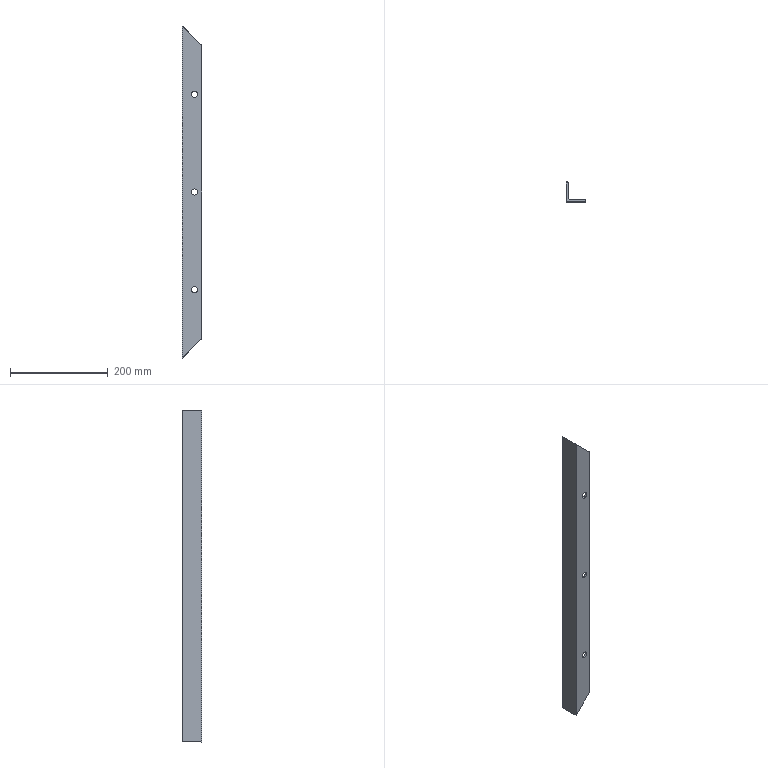Part | SolidWorks | features ICE 2, Extrusion 1 | 1 solid | 17 faces | box 40 x 40 x 680 mm | volume 199359 mm3 | cylinder 9 | plane 8 | commonest cylinder face diameters 13 x6 4 x2 8 x1
STEP:
#1=CARTESIAN_POINT('',(31.5,0.,540.));
#2=VERTEX_POINT('',#1);
#3=CARTESIAN_POINT('',(18.5,0.,540.));
#4=VERTEX_POINT('',#3);
#5=CARTESIAN_POINT('',(25.,0.,540.));
#6=DIRECTION('',(0.,1.,0.));
#7=DIRECTION('',(0.,0.,1.));
#8=AXIS2_PLACEMENT_3D('',#5,#6,#7);
#9=CIRCLE('',#8,6.5);
#10=EDGE_CURVE('',#2,#4,#9,.T.);
#11=ORIENTED_EDGE('',*,*,#10,.F.);
#12=CARTESIAN_POINT('',(31.5,4.,540.));
#13=VERTEX_POINT('',#12);
#14=CARTESIAN_POINT('',(31.5,-6.,540.));
#15=DIRECTION('',(0.,1.,0.));
#16=VECTOR('',#15,1000.);
#17=LINE('',#14,#16);
#18=EDGE_CURVE('',#2,#13,#17,.T.);
#19=ORIENTED_EDGE('',*,*,#18,.T.);
#20=CARTESIAN_POINT('',(18.5,4.,540.));
#21=VERTEX_POINT('',#20);
#22=CARTESIAN_POINT('',(25.,4.,540.));
#23=DIRECTION('',(0.,1.,0.));
#24=DIRECTION('',(-1.,0.,0.));
#25=AXIS2_PLACEMENT_3D('',#22,#23,#24);
#26=CIRCLE('',#25,6.5);
#27=EDGE_CURVE('',#13,#21,#26,.T.);
#28=ORIENTED_EDGE('',*,*,#27,.T.);
#29=CARTESIAN_POINT('',(18.5,-6.,540.));
#30=DIRECTION('',(0.,1.,0.));
#31=VECTOR('',#30,1000.);
#32=LINE('',#29,#31);
#33=EDGE_CURVE('',#4,#21,#32,.T.);
#34=ORIENTED_EDGE('',*,*,#33,.F.);
#35=EDGE_LOOP('',(#11,#19,#28,#34));
#36=FACE_OUTER_BOUND('',#35,.T.);
#37=CARTESIAN_POINT('',(25.,-6.,540.));
#38=DIRECTION('',(0.,1.,0.));
#39=DIRECTION('',(-1.,0.,0.));
#40=AXIS2_PLACEMENT_3D('',#37,#38,#39);
#41=CYLINDRICAL_SURFACE('',#40,6.5);
#42=ADVANCED_FACE('',(#36),#41,.F.);
#43=CARTESIAN_POINT('',(31.5,0.,340.));
#44=VERTEX_POINT('',#43);
#45=CARTESIAN_POINT('',(18.5,0.,340.));
#46=VERTEX_POINT('',#45);
#47=CARTESIAN_POINT('',(25.,0.,340.));
#48=DIRECTION('',(0.,1.,0.));
#49=DIRECTION('',(0.,0.,1.));
#50=AXIS2_PLACEMENT_3D('',#47,#48,#49);
#51=CIRCLE('',#50,6.5);
#52=EDGE_CURVE('',#44,#46,#51,.T.);
#53=ORIENTED_EDGE('',*,*,#52,.F.);
#54=CARTESIAN_POINT('',(31.5,4.,340.));
#55=VERTEX_POINT('',#54);
#56=CARTESIAN_POINT('',(31.5,-6.,340.));
#57=DIRECTION('',(0.,1.,0.));
#58=VECTOR('',#57,1000.);
#59=LINE('',#56,#58);
#60=EDGE_CURVE('',#44,#55,#59,.T.);
#61=ORIENTED_EDGE('',*,*,#60,.T.);
#62=CARTESIAN_POINT('',(18.5,4.,340.));
#63=VERTEX_POINT('',#62);
#64=CARTESIAN_POINT('',(25.,4.,340.));
#65=DIRECTION('',(0.,1.,0.));
#66=DIRECTION('',(-1.,0.,0.));
#67=AXIS2_PLACEMENT_3D('',#64,#65,#66);
#68=CIRCLE('',#67,6.5);
#69=EDGE_CURVE('',#55,#63,#68,.T.);
#70=ORIENTED_EDGE('',*,*,#69,.T.);
#71=CARTESIAN_POINT('',(18.5,-6.,340.));
#72=DIRECTION('',(0.,1.,0.));
#73=VECTOR('',#72,1000.);
#74=LINE('',#71,#73);
#75=EDGE_CURVE('',#46,#63,#74,.T.);
#76=ORIENTED_EDGE('',*,*,#75,.F.);
#77=EDGE_LOOP('',(#53,#61,#70,#76));
#78=FACE_OUTER_BOUND('',#77,.T.);
#79=CARTESIAN_POINT('',(25.,-6.,340.));
#80=DIRECTION('',(0.,1.,0.));
#81=DIRECTION('',(-1.,0.,0.));
#82=AXIS2_PLACEMENT_3D('',#79,#80,#81);
#83=CYLINDRICAL_SURFACE('',#82,6.5);
#84=ADVANCED_FACE('',(#78),#83,.F.);
#85=CARTESIAN_POINT('',(31.5,0.,140.));
#86=VERTEX_POINT('',#85);
#87=CARTESIAN_POINT('',(18.5,0.,140.));
#88=VERTEX_POINT('',#87);
#89=CARTESIAN_POINT('',(25.,0.,140.));
#90=DIRECTION('',(0.,1.,0.));
#91=DIRECTION('',(0.,0.,1.));
#92=AXIS2_PLACEMENT_3D('',#89,#90,#91);
#93=CIRCLE('',#92,6.5);
#94=EDGE_CURVE('',#86,#88,#93,.T.);
#95=ORIENTED_EDGE('',*,*,#94,.F.);
#96=CARTESIAN_POINT('',(31.5,4.,140.));
#97=VERTEX_POINT('',#96);
#98=CARTESIAN_POINT('',(31.5,-6.,140.));
#99=DIRECTION('',(0.,1.,0.));
#100=VECTOR('',#99,1000.);
#101=LINE('',#98,#100);
#102=EDGE_CURVE('',#86,#97,#101,.T.);
#103=ORIENTED_EDGE('',*,*,#102,.T.);
#104=CARTESIAN_POINT('',(18.5,4.,140.));
#105=VERTEX_POINT('',#104);
#106=CARTESIAN_POINT('',(25.,4.,140.));
#107=DIRECTION('',(0.,1.,0.));
#108=DIRECTION('',(-1.,0.,0.));
#109=AXIS2_PLACEMENT_3D('',#106,#107,#108);
#110=CIRCLE('',#109,6.5);
#111=EDGE_CURVE('',#97,#105,#110,.T.);
#112=ORIENTED_EDGE('',*,*,#111,.T.);
#113=CARTESIAN_POINT('',(18.5,-6.,140.));
#114=DIRECTION('',(0.,1.,0.));
#115=VECTOR('',#114,1000.);
#116=LINE('',#113,#115);
#117=EDGE_CURVE('',#88,#105,#116,.T.);
#118=ORIENTED_EDGE('',*,*,#117,.F.);
#119=EDGE_LOOP('',(#95,#103,#112,#118));
#120=FACE_OUTER_BOUND('',#119,.T.);
#121=CARTESIAN_POINT('',(25.,-6.,140.));
#122=DIRECTION('',(0.,1.,0.));
#123=DIRECTION('',(-1.,0.,0.));
#124=AXIS2_PLACEMENT_3D('',#121,#122,#123);
#125=CYLINDRICAL_SURFACE('',#124,6.5);
#126=ADVANCED_FACE('',(#120),#125,.F.);
#127=CARTESIAN_POINT('',(0.,40.,680.));
#128=VERTEX_POINT('',#127);
#129=CARTESIAN_POINT('',(0.,40.,0.));
#130=VERTEX_POINT('',#129);
#131=CARTESIAN_POINT('',(0.,40.,680.));
#132=DIRECTION('',(0.,0.,-1.));
#133=VECTOR('',#132,1000.);
#134=LINE('',#131,#133);
#135=EDGE_CURVE('',#128,#130,#134,.T.);
#136=ORIENTED_EDGE('',*,*,#135,.F.);
#137=CARTESIAN_POINT('',(2.,40.,678.));
#138=VERTEX_POINT('',#137);
#139=CARTESIAN_POINT('',(40.,40.,640.));
#140=DIRECTION('',(-0.7071,0.,0.7071));
#141=VECTOR('',#140,1000.);
#142=LINE('',#139,#141);
#143=EDGE_CURVE('',#138,#128,#142,.T.);
#144=ORIENTED_EDGE('',*,*,#143,.F.);
#145=CARTESIAN_POINT('',(2.,40.,2.));
#146=VERTEX_POINT('',#145);
#147=CARTESIAN_POINT('',(2.,40.,680.));
#148=DIRECTION('',(0.,0.,-1.));
#149=VECTOR('',#148,1000.);
#150=LINE('',#147,#149);
#151=EDGE_CURVE('',#138,#146,#150,.T.);
#152=ORIENTED_EDGE('',*,*,#151,.T.);
#153=CARTESIAN_POINT('',(0.,40.,0.));
#154=DIRECTION('',(0.7071,0.,0.7071));
#155=VECTOR('',#154,1000.);
#156=LINE('',#153,#155);
#157=EDGE_CURVE('',#130,#146,#156,.T.);
#158=ORIENTED_EDGE('',*,*,#157,.F.);
#159=EDGE_LOOP('',(#136,#144,#152,#158));
#160=FACE_OUTER_BOUND('',#159,.T.);
#161=CARTESIAN_POINT('',(2.,40.,680.));
#162=DIRECTION('',(0.,-1.,0.));
#163=DIRECTION('',(0.,0.,-1.));
#164=AXIS2_PLACEMENT_3D('',#161,#162,#163);
#165=PLANE('',#164);
#166=ADVANCED_FACE('',(#160),#165,.F.);
#167=CARTESIAN_POINT('',(0.,0.,0.));
#168=VERTEX_POINT('',#167);
#169=CARTESIAN_POINT('',(0.,40.,0.));
#170=DIRECTION('',(0.,-1.,0.));
#171=VECTOR('',#170,1000.);
#172=LINE('',#169,#171);
#173=EDGE_CURVE('',#130,#168,#172,.T.);
#174=ORIENTED_EDGE('',*,*,#173,.T.);
#175=CARTESIAN_POINT('',(0.,0.,680.));
#176=VERTEX_POINT('',#175);
#177=CARTESIAN_POINT('',(0.,0.,680.));
#178=DIRECTION('',(0.,0.,-1.));
#179=VECTOR('',#178,1000.);
#180=LINE('',#177,#179);
#181=EDGE_CURVE('',#176,#168,#180,.T.);
#182=ORIENTED_EDGE('',*,*,#181,.F.);
#183=CARTESIAN_POINT('',(0.,40.,680.));
#184=DIRECTION('',(0.,-1.,0.));
#185=VECTOR('',#184,1000.);
#186=LINE('',#183,#185);
#187=EDGE_CURVE('',#128,#176,#186,.T.);
#188=ORIENTED_EDGE('',*,*,#187,.F.);
#189=ORIENTED_EDGE('',*,*,#135,.T.);
#190=EDGE_LOOP('',(#174,#182,#188,#189));
#191=FACE_OUTER_BOUND('',#190,.T.);
#192=CARTESIAN_POINT('',(0.,40.,680.));
#193=DIRECTION('',(1.,0.,0.));
#194=DIRECTION('',(0.,1.,0.));
#195=AXIS2_PLACEMENT_3D('',#192,#193,#194);
#196=PLANE('',#195);
#197=ADVANCED_FACE('',(#191),#196,.F.);
#198=CARTESIAN_POINT('',(25.,0.,540.));
#199=DIRECTION('',(0.,1.,0.));
#200=DIRECTION('',(0.,0.,1.));
#201=AXIS2_PLACEMENT_3D('',#198,#199,#200);
#202=CIRCLE('',#201,6.5);
#203=EDGE_CURVE('',#4,#2,#202,.T.);
#204=ORIENTED_EDGE('',*,*,#203,.T.);
#205=ORIENTED_EDGE('',*,*,#10,.T.);
#206=EDGE_LOOP('',(#204,#205));
#207=FACE_BOUND('',#206,.T.);
#208=CARTESIAN_POINT('',(25.,0.,340.));
#209=DIRECTION('',(0.,1.,0.));
#210=DIRECTION('',(0.,0.,1.));
#211=AXIS2_PLACEMENT_3D('',#208,#209,#210);
#212=CIRCLE('',#211,6.5);
#213=EDGE_CURVE('',#46,#44,#212,.T.);
#214=ORIENTED_EDGE('',*,*,#213,.T.);
#215=ORIENTED_EDGE('',*,*,#52,.T.);
#216=EDGE_LOOP('',(#214,#215));
#217=FACE_BOUND('',#216,.T.);
#218=CARTESIAN_POINT('',(25.,0.,140.));
#219=DIRECTION('',(0.,1.,0.));
#220=DIRECTION('',(0.,0.,1.));
#221=AXIS2_PLACEMENT_3D('',#218,#219,#220);
#222=CIRCLE('',#221,6.5);
#223=EDGE_CURVE('',#88,#86,#222,.T.);
#224=ORIENTED_EDGE('',*,*,#223,.T.);
#225=ORIENTED_EDGE('',*,*,#94,.T.);
#226=EDGE_LOOP('',(#224,#225));
#227=FACE_BOUND('',#226,.T.);
#228=CARTESIAN_POINT('',(40.,0.,640.));
#229=VERTEX_POINT('',#228);
#230=CARTESIAN_POINT('',(40.,0.,40.));
#231=VERTEX_POINT('',#230);
#232=CARTESIAN_POINT('',(40.,0.,680.));
#233=DIRECTION('',(0.,0.,-1.));
#234=VECTOR('',#233,1000.);
#235=LINE('',#232,#234);
#236=EDGE_CURVE('',#229,#231,#235,.T.);
#237=ORIENTED_EDGE('',*,*,#236,.F.);
#238=CARTESIAN_POINT('',(40.,0.,640.));
#239=DIRECTION('',(-0.7071,0.,0.7071));
#240=VECTOR('',#239,1000.);
#241=LINE('',#238,#240);
#242=EDGE_CURVE('',#229,#176,#241,.T.);
#243=ORIENTED_EDGE('',*,*,#242,.T.);
#244=ORIENTED_EDGE('',*,*,#181,.T.);
#245=CARTESIAN_POINT('',(0.,0.,0.));
#246=DIRECTION('',(0.7071,0.,0.7071));
#247=VECTOR('',#246,1000.);
#248=LINE('',#245,#247);
#249=EDGE_CURVE('',#168,#231,#248,.T.);
#250=ORIENTED_EDGE('',*,*,#249,.T.);
#251=EDGE_LOOP('',(#237,#243,#244,#250));
#252=FACE_OUTER_BOUND('',#251,.T.);
#253=CARTESIAN_POINT('',(0.,0.,680.));
#254=DIRECTION('',(0.,1.,0.));
#255=DIRECTION('',(0.,0.,1.));
#256=AXIS2_PLACEMENT_3D('',#253,#254,#255);
#257=PLANE('',#256);
#258=ADVANCED_FACE('',(#207,#217,#227,#252),#257,.F.);
#259=CARTESIAN_POINT('',(40.,2.,640.));
#260=VERTEX_POINT('',#259);
#261=CARTESIAN_POINT('',(40.,2.,40.));
#262=VERTEX_POINT('',#261);
#263=CARTESIAN_POINT('',(40.,2.,680.));
#264=DIRECTION('',(0.,0.,-1.));
#265=VECTOR('',#264,1000.);
#266=LINE('',#263,#265);
#267=EDGE_CURVE('',#260,#262,#266,.T.);
#268=ORIENTED_EDGE('',*,*,#267,.F.);
#269=CARTESIAN_POINT('',(40.,0.,640.));
#270=DIRECTION('',(0.,1.,0.));
#271=VECTOR('',#270,1000.);
#272=LINE('',#269,#271);
#273=EDGE_CURVE('',#229,#260,#272,.T.);
#274=ORIENTED_EDGE('',*,*,#273,.F.);
#275=ORIENTED_EDGE('',*,*,#236,.T.);
#276=CARTESIAN_POINT('',(40.,0.,40.));
#277=DIRECTION('',(0.,1.,0.));
#278=VECTOR('',#277,1000.);
#279=LINE('',#276,#278);
#280=EDGE_CURVE('',#231,#262,#279,.T.);
#281=ORIENTED_EDGE('',*,*,#280,.T.);
#282=EDGE_LOOP('',(#268,#274,#275,#281));
#283=FACE_OUTER_BOUND('',#282,.T.);
#284=CARTESIAN_POINT('',(40.,0.,680.));
#285=DIRECTION('',(-1.,0.,0.));
#286=DIRECTION('',(0.,0.,1.));
#287=AXIS2_PLACEMENT_3D('',#284,#285,#286);
#288=PLANE('',#287);
#289=ADVANCED_FACE('',(#283),#288,.F.);
#290=CARTESIAN_POINT('',(38.,4.,642.));
#291=VERTEX_POINT('',#290);
#292=CARTESIAN_POINT('',(38.,4.,38.));
#293=VERTEX_POINT('',#292);
#294=CARTESIAN_POINT('',(38.,4.,680.));
#295=DIRECTION('',(0.,0.,-1.));
#296=VECTOR('',#295,1000.);
#297=LINE('',#294,#296);
#298=EDGE_CURVE('',#291,#293,#297,.T.);
#299=ORIENTED_EDGE('',*,*,#298,.F.);
#300=CARTESIAN_POINT('',(38.,4.,642.));
#301=CARTESIAN_POINT('',(39.172,4.,640.828));
#302=CARTESIAN_POINT('',(40.,3.172,640.));
#303=CARTESIAN_POINT('',(40.,2.,640.));
#304=(BOUNDED_CURVE()B_SPLINE_CURVE(3,(#300,#301,#302,#303),.UNSPECIFIED.,.F.,.F.)B_SPLINE_CURVE_WITH_KNOTS((4,4),(4.712,6.283),.UNSPECIFIED.)CURVE()GEOMETRIC_REPRESENTATION_ITEM()RATIONAL_B_SPLINE_CURVE((1.,0.8047,0.8047,1.))REPRESENTATION_ITEM(''));
#305=EDGE_CURVE('',#291,#260,#304,.T.);
#306=ORIENTED_EDGE('',*,*,#305,.T.);
#307=ORIENTED_EDGE('',*,*,#267,.T.);
#308=CARTESIAN_POINT('',(40.,2.,40.));
#309=CARTESIAN_POINT('',(40.,3.172,40.));
#310=CARTESIAN_POINT('',(39.172,4.,39.172));
#311=CARTESIAN_POINT('',(38.,4.,38.));
#312=(BOUNDED_CURVE()B_SPLINE_CURVE(3,(#308,#309,#310,#311),.UNSPECIFIED.,.F.,.F.)B_SPLINE_CURVE_WITH_KNOTS((4,4),(3.142,4.712),.UNSPECIFIED.)CURVE()GEOMETRIC_REPRESENTATION_ITEM()RATIONAL_B_SPLINE_CURVE((1.,0.8047,0.8047,1.))REPRESENTATION_ITEM(''));
#313=EDGE_CURVE('',#262,#293,#312,.T.);
#314=ORIENTED_EDGE('',*,*,#313,.T.);
#315=EDGE_LOOP('',(#299,#306,#307,#314));
#316=FACE_OUTER_BOUND('',#315,.T.);
#317=CARTESIAN_POINT('',(38.,2.,680.));
#318=DIRECTION('',(0.,0.,-1.));
#319=DIRECTION('',(-1.,0.,0.));
#320=AXIS2_PLACEMENT_3D('',#317,#318,#319);
#321=CYLINDRICAL_SURFACE('',#320,2.);
#322=ADVANCED_FACE('',(#316),#321,.T.);
#323=CARTESIAN_POINT('',(25.,4.,540.));
#324=DIRECTION('',(0.,1.,0.));
#325=DIRECTION('',(-1.,0.,0.));
#326=AXIS2_PLACEMENT_3D('',#323,#324,#325);
#327=CIRCLE('',#326,6.5);
#328=EDGE_CURVE('',#21,#13,#327,.T.);
#329=ORIENTED_EDGE('',*,*,#328,.F.);
#330=ORIENTED_EDGE('',*,*,#27,.F.);
#331=EDGE_LOOP('',(#329,#330));
#332=FACE_BOUND('',#331,.T.);
#333=CARTESIAN_POINT('',(25.,4.,340.));
#334=DIRECTION('',(0.,1.,0.));
#335=DIRECTION('',(-1.,0.,0.));
#336=AXIS2_PLACEMENT_3D('',#333,#334,#335);
#337=CIRCLE('',#336,6.5);
#338=EDGE_CURVE('',#63,#55,#337,.T.);
#339=ORIENTED_EDGE('',*,*,#338,.F.);
#340=ORIENTED_EDGE('',*,*,#69,.F.);
#341=EDGE_LOOP('',(#339,#340));
#342=FACE_BOUND('',#341,.T.);
#343=CARTESIAN_POINT('',(25.,4.,140.));
#344=DIRECTION('',(0.,1.,0.));
#345=DIRECTION('',(-1.,0.,0.));
#346=AXIS2_PLACEMENT_3D('',#343,#344,#345);
#347=CIRCLE('',#346,6.5);
#348=EDGE_CURVE('',#105,#97,#347,.T.);
#349=ORIENTED_EDGE('',*,*,#348,.F.);
#350=ORIENTED_EDGE('',*,*,#111,.F.);
#351=EDGE_LOOP('',(#349,#350));
#352=FACE_BOUND('',#351,.T.);
#353=CARTESIAN_POINT('',(8.,4.,672.));
#354=VERTEX_POINT('',#353);
#355=CARTESIAN_POINT('',(8.,4.,8.));
#356=VERTEX_POINT('',#355);
#357=CARTESIAN_POINT('',(8.,4.,680.));
#358=DIRECTION('',(0.,0.,-1.));
#359=VECTOR('',#358,1000.);
#360=LINE('',#357,#359);
#361=EDGE_CURVE('',#354,#356,#360,.T.);
#362=ORIENTED_EDGE('',*,*,#361,.F.);
#363=CARTESIAN_POINT('',(19.,4.,661.));
#364=DIRECTION('',(0.7071,0.,-0.7071));
#365=VECTOR('',#364,1000.);
#366=LINE('',#363,#365);
#367=EDGE_CURVE('',#354,#291,#366,.T.);
#368=ORIENTED_EDGE('',*,*,#367,.T.);
#369=ORIENTED_EDGE('',*,*,#298,.T.);
#370=CARTESIAN_POINT('',(359.,4.,359.));
#371=DIRECTION('',(-0.7071,0.,-0.7071));
#372=VECTOR('',#371,1000.);
#373=LINE('',#370,#372);
#374=EDGE_CURVE('',#293,#356,#373,.T.);
#375=ORIENTED_EDGE('',*,*,#374,.T.);
#376=EDGE_LOOP('',(#362,#368,#369,#375));
#377=FACE_OUTER_BOUND('',#376,.T.);
#378=CARTESIAN_POINT('',(38.,4.,680.));
#379=DIRECTION('',(0.,-1.,0.));
#380=DIRECTION('',(1.,0.,0.));
#381=AXIS2_PLACEMENT_3D('',#378,#379,#380);
#382=PLANE('',#381);
#383=ADVANCED_FACE('',(#332,#342,#352,#377),#382,.F.);
#384=CARTESIAN_POINT('',(4.,8.,676.));
#385=VERTEX_POINT('',#384);
#386=CARTESIAN_POINT('',(4.,8.,4.));
#387=VERTEX_POINT('',#386);
#388=CARTESIAN_POINT('',(4.,8.,680.));
#389=DIRECTION('',(0.,0.,-1.));
#390=VECTOR('',#389,1000.);
#391=LINE('',#388,#390);
#392=EDGE_CURVE('',#385,#387,#391,.T.);
#393=ORIENTED_EDGE('',*,*,#392,.F.);
#394=CARTESIAN_POINT('',(4.,8.,676.));
#395=CARTESIAN_POINT('',(4.,5.657,676.));
#396=CARTESIAN_POINT('',(5.657,4.,674.343));
#397=CARTESIAN_POINT('',(8.,4.,672.));
#398=(BOUNDED_CURVE()B_SPLINE_CURVE(3,(#394,#395,#396,#397),.UNSPECIFIED.,.F.,.F.)B_SPLINE_CURVE_WITH_KNOTS((4,4),(3.142,4.712),.UNSPECIFIED.)CURVE()GEOMETRIC_REPRESENTATION_ITEM()RATIONAL_B_SPLINE_CURVE((1.,0.8047,0.8047,1.))REPRESENTATION_ITEM(''));
#399=EDGE_CURVE('',#385,#354,#398,.T.);
#400=ORIENTED_EDGE('',*,*,#399,.T.);
#401=ORIENTED_EDGE('',*,*,#361,.T.);
#402=CARTESIAN_POINT('',(8.,4.,8.));
#403=CARTESIAN_POINT('',(5.657,4.,5.657));
#404=CARTESIAN_POINT('',(4.,5.657,4.));
#405=CARTESIAN_POINT('',(4.,8.,4.));
#406=(BOUNDED_CURVE()B_SPLINE_CURVE(3,(#402,#403,#404,#405),.UNSPECIFIED.,.F.,.F.)B_SPLINE_CURVE_WITH_KNOTS((4,4),(4.712,6.283),.UNSPECIFIED.)CURVE()GEOMETRIC_REPRESENTATION_ITEM()RATIONAL_B_SPLINE_CURVE((1.,0.8047,0.8047,1.))REPRESENTATION_ITEM(''));
#407=EDGE_CURVE('',#356,#387,#406,.T.);
#408=ORIENTED_EDGE('',*,*,#407,.T.);
#409=EDGE_LOOP('',(#393,#400,#401,#408));
#410=FACE_OUTER_BOUND('',#409,.T.);
#411=CARTESIAN_POINT('',(8.,8.,680.));
#412=DIRECTION('',(0.,0.,-1.));
#413=DIRECTION('',(-1.,0.,0.));
#414=AXIS2_PLACEMENT_3D('',#411,#412,#413);
#415=CYLINDRICAL_SURFACE('',#414,4.);
#416=ADVANCED_FACE('',(#410),#415,.F.);
#417=CARTESIAN_POINT('',(4.,38.,676.));
#418=VERTEX_POINT('',#417);
#419=CARTESIAN_POINT('',(4.,38.,4.));
#420=VERTEX_POINT('',#419);
#421=CARTESIAN_POINT('',(4.,38.,680.));
#422=DIRECTION('',(0.,0.,-1.));
#423=VECTOR('',#422,1000.);
#424=LINE('',#421,#423);
#425=EDGE_CURVE('',#418,#420,#424,.T.);
#426=ORIENTED_EDGE('',*,*,#425,.F.);
#427=CARTESIAN_POINT('',(4.,8.,676.));
#428=DIRECTION('',(0.,-1.,0.));
#429=VECTOR('',#428,1000.);
#430=LINE('',#427,#429);
#431=EDGE_CURVE('',#418,#385,#430,.T.);
#432=ORIENTED_EDGE('',*,*,#431,.T.);
#433=ORIENTED_EDGE('',*,*,#392,.T.);
#434=CARTESIAN_POINT('',(4.,8.,4.));
#435=DIRECTION('',(0.,1.,0.));
#436=VECTOR('',#435,1000.);
#437=LINE('',#434,#436);
#438=EDGE_CURVE('',#387,#420,#437,.T.);
#439=ORIENTED_EDGE('',*,*,#438,.T.);
#440=EDGE_LOOP('',(#426,#432,#433,#439));
#441=FACE_OUTER_BOUND('',#440,.T.);
#442=CARTESIAN_POINT('',(4.,8.,680.));
#443=DIRECTION('',(-1.,0.,0.));
#444=DIRECTION('',(0.,-1.,0.));
#445=AXIS2_PLACEMENT_3D('',#442,#443,#444);
#446=PLANE('',#445);
#447=ADVANCED_FACE('',(#441),#446,.F.);
#448=ORIENTED_EDGE('',*,*,#151,.F.);
#449=CARTESIAN_POINT('',(2.,40.,678.));
#450=CARTESIAN_POINT('',(3.172,40.,676.828));
#451=CARTESIAN_POINT('',(4.,39.172,676.));
#452=CARTESIAN_POINT('',(4.,38.,676.));
#453=(BOUNDED_CURVE()B_SPLINE_CURVE(3,(#449,#450,#451,#452),.UNSPECIFIED.,.F.,.T.)B_SPLINE_CURVE_WITH_KNOTS((4,4),(4.712,6.283),.UNSPECIFIED.)CURVE()GEOMETRIC_REPRESENTATION_ITEM()RATIONAL_B_SPLINE_CURVE((1.,0.8047,0.8047,1.))REPRESENTATION_ITEM(''));
#454=EDGE_CURVE('',#138,#418,#453,.T.);
#455=ORIENTED_EDGE('',*,*,#454,.T.);
#456=ORIENTED_EDGE('',*,*,#425,.T.);
#457=CARTESIAN_POINT('',(4.,38.,4.));
#458=CARTESIAN_POINT('',(4.,39.172,4.));
#459=CARTESIAN_POINT('',(3.172,40.,3.172));
#460=CARTESIAN_POINT('',(2.,40.,2.));
#461=(BOUNDED_CURVE()B_SPLINE_CURVE(3,(#457,#458,#459,#460),.UNSPECIFIED.,.F.,.F.)B_SPLINE_CURVE_WITH_KNOTS((4,4),(3.142,4.712),.UNSPECIFIED.)CURVE()GEOMETRIC_REPRESENTATION_ITEM()RATIONAL_B_SPLINE_CURVE((1.,0.8047,0.8047,1.))REPRESENTATION_ITEM(''));
#462=EDGE_CURVE('',#420,#146,#461,.T.);
#463=ORIENTED_EDGE('',*,*,#462,.T.);
#464=EDGE_LOOP('',(#448,#455,#456,#463));
#465=FACE_OUTER_BOUND('',#464,.T.);
#466=CARTESIAN_POINT('',(2.,38.,680.));
#467=DIRECTION('',(0.,0.,-1.));
#468=DIRECTION('',(-1.,0.,0.));
#469=AXIS2_PLACEMENT_3D('',#466,#467,#468);
#470=CYLINDRICAL_SURFACE('',#469,2.);
#471=ADVANCED_FACE('',(#465),#470,.T.);
#472=ORIENTED_EDGE('',*,*,#280,.F.);
#473=ORIENTED_EDGE('',*,*,#249,.F.);
#474=ORIENTED_EDGE('',*,*,#173,.F.);
#475=ORIENTED_EDGE('',*,*,#157,.T.);
#476=ORIENTED_EDGE('',*,*,#462,.F.);
#477=ORIENTED_EDGE('',*,*,#438,.F.);
#478=ORIENTED_EDGE('',*,*,#407,.F.);
#479=ORIENTED_EDGE('',*,*,#374,.F.);
#480=ORIENTED_EDGE('',*,*,#313,.F.);
#481=EDGE_LOOP('',(#472,#473,#474,#475,#476,#477,#478,#479,#480));
#482=FACE_OUTER_BOUND('',#481,.T.);
#483=CARTESIAN_POINT('',(0.,0.,0.));
#484=DIRECTION('',(-0.7071,0.,0.7071));
#485=DIRECTION('',(0.7071,0.,0.7071));
#486=AXIS2_PLACEMENT_3D('',#483,#484,#485);
#487=PLANE('',#486);
#488=ADVANCED_FACE('',(#482),#487,.F.);
#489=ORIENTED_EDGE('',*,*,#367,.F.);
#490=ORIENTED_EDGE('',*,*,#399,.F.);
#491=ORIENTED_EDGE('',*,*,#431,.F.);
#492=ORIENTED_EDGE('',*,*,#454,.F.);
#493=ORIENTED_EDGE('',*,*,#143,.T.);
#494=ORIENTED_EDGE('',*,*,#187,.T.);
#495=ORIENTED_EDGE('',*,*,#242,.F.);
#496=ORIENTED_EDGE('',*,*,#273,.T.);
#497=ORIENTED_EDGE('',*,*,#305,.F.);
#498=EDGE_LOOP('',(#489,#490,#491,#492,#493,#494,#495,#496,#497));
#499=FACE_OUTER_BOUND('',#498,.T.);
#500=CARTESIAN_POINT('',(40.,0.,640.));
#501=DIRECTION('',(-0.7071,0.,-0.7071));
#502=DIRECTION('',(-0.7071,0.,0.7071));
#503=AXIS2_PLACEMENT_3D('',#500,#501,#502);
#504=PLANE('',#503);
#505=ADVANCED_FACE('',(#499),#504,.F.);
#506=ORIENTED_EDGE('',*,*,#102,.F.);
#507=ORIENTED_EDGE('',*,*,#223,.F.);
#508=ORIENTED_EDGE('',*,*,#117,.T.);
#509=ORIENTED_EDGE('',*,*,#348,.T.);
#510=EDGE_LOOP('',(#506,#507,#508,#509));
#511=FACE_OUTER_BOUND('',#510,.T.);
#512=CARTESIAN_POINT('',(25.,-6.,140.));
#513=DIRECTION('',(0.,1.,0.));
#514=DIRECTION('',(-1.,0.,0.));
#515=AXIS2_PLACEMENT_3D('',#512,#513,#514);
#516=CYLINDRICAL_SURFACE('',#515,6.5);
#517=ADVANCED_FACE('',(#511),#516,.F.);
#518=ORIENTED_EDGE('',*,*,#60,.F.);
#519=ORIENTED_EDGE('',*,*,#213,.F.);
#520=ORIENTED_EDGE('',*,*,#75,.T.);
#521=ORIENTED_EDGE('',*,*,#338,.T.);
#522=EDGE_LOOP('',(#518,#519,#520,#521));
#523=FACE_OUTER_BOUND('',#522,.T.);
#524=CARTESIAN_POINT('',(25.,-6.,340.));
#525=DIRECTION('',(0.,1.,0.));
#526=DIRECTION('',(-1.,0.,0.));
#527=AXIS2_PLACEMENT_3D('',#524,#525,#526);
#528=CYLINDRICAL_SURFACE('',#527,6.5);
#529=ADVANCED_FACE('',(#523),#528,.F.);
#530=ORIENTED_EDGE('',*,*,#18,.F.);
#531=ORIENTED_EDGE('',*,*,#203,.F.);
#532=ORIENTED_EDGE('',*,*,#33,.T.);
#533=ORIENTED_EDGE('',*,*,#328,.T.);
#534=EDGE_LOOP('',(#530,#531,#532,#533));
#535=FACE_OUTER_BOUND('',#534,.T.);
#536=CARTESIAN_POINT('',(25.,-6.,540.));
#537=DIRECTION('',(0.,1.,0.));
#538=DIRECTION('',(-1.,0.,0.));
#539=AXIS2_PLACEMENT_3D('',#536,#537,#538);
#540=CYLINDRICAL_SURFACE('',#539,6.5);
#541=ADVANCED_FACE('',(#535),#540,.F.);
#542=CLOSED_SHELL('',(#42,#84,#126,#166,#197,#258,#289,#322,#383,#416,#447,#471,#488,#505,#517,#529,#541));
#543=MANIFOLD_SOLID_BREP('',#542);
#544=CARTESIAN_POINT('',(0.,0.,0.));
#545=DIRECTION('',(0.,0.,1.));
#546=DIRECTION('',(1.,0.,0.));
#547=AXIS2_PLACEMENT_3D('',#544,#545,#546);
#548=(LENGTH_UNIT()NAMED_UNIT(*)SI_UNIT(.MILLI.,.METRE.));
#549=UNCERTAINTY_MEASURE_WITH_UNIT(LENGTH_MEASURE(0.00001),#548,'','');
#550=(NAMED_UNIT(*)PLANE_ANGLE_UNIT()SI_UNIT($,.RADIAN.));
#551=(NAMED_UNIT(*)SI_UNIT($,.STERADIAN.)SOLID_ANGLE_UNIT());
#552=(GEOMETRIC_REPRESENTATION_CONTEXT(3)GLOBAL_UNCERTAINTY_ASSIGNED_CONTEXT((#549))GLOBAL_UNIT_ASSIGNED_CONTEXT((#548,#550,#551))REPRESENTATION_CONTEXT('',''));
#553=ADVANCED_BREP_SHAPE_REPRESENTATION('',(#543,#547),#552);